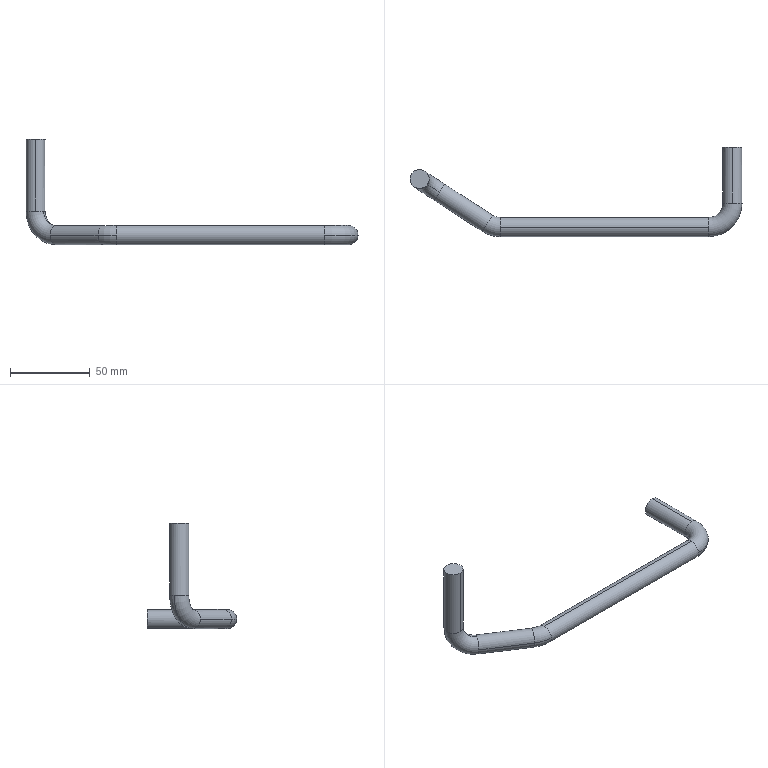Part | SolidWorks | features 3DProfileFeature 2, Sweep 1 | 1 solid | 16 faces | box 208.199 x 56 x 66 mm | volume 34151 mm3 | cylinder 8 | torus 6 | plane 2 | commonest cylinder face diameters 12 x8
STEP:
#1=CARTESIAN_POINT('',(-33.619,21.831,-6.));
#2=VERTEX_POINT('',#1);
#3=CARTESIAN_POINT('',(-30.351,26.863,0.));
#4=VERTEX_POINT('',#3);
#5=CARTESIAN_POINT('',(-33.619,21.831,0.));
#6=DIRECTION('',(0.8387,-0.5446,0.));
#7=DIRECTION('',(0.4568,0.7034,-0.5446));
#8=AXIS2_PLACEMENT_3D('',#5,#6,#7);
#9=CIRCLE('',#8,6.);
#10=EDGE_CURVE('',#2,#4,#9,.T.);
#11=ORIENTED_EDGE('',*,*,#10,.F.);
#12=CARTESIAN_POINT('',(-51.231,33.268,15.));
#13=VERTEX_POINT('',#12);
#14=CARTESIAN_POINT('',(-33.619,21.831,15.));
#15=DIRECTION('',(0.5446,0.8387,0.));
#16=DIRECTION('',(-0.8387,0.5446,0.));
#17=AXIS2_PLACEMENT_3D('',#14,#15,#16);
#18=CIRCLE('',#17,21.);
#19=EDGE_CURVE('',#2,#13,#18,.T.);
#20=ORIENTED_EDGE('',*,*,#19,.T.);
#21=CARTESIAN_POINT('',(-46.199,36.,15.));
#22=VERTEX_POINT('',#21);
#23=CARTESIAN_POINT('',(-46.199,30.,15.));
#24=DIRECTION('',(0.,0.,-1.));
#25=DIRECTION('',(0.,1.,0.));
#26=AXIS2_PLACEMENT_3D('',#23,#24,#25);
#27=CIRCLE('',#26,6.);
#28=EDGE_CURVE('',#13,#22,#27,.T.);
#29=ORIENTED_EDGE('',*,*,#28,.T.);
#30=CARTESIAN_POINT('',(-41.167,26.732,15.));
#31=VERTEX_POINT('',#30);
#32=CARTESIAN_POINT('',(-46.199,30.,15.));
#33=DIRECTION('',(0.,0.,-1.));
#34=DIRECTION('',(0.,1.,0.));
#35=AXIS2_PLACEMENT_3D('',#32,#33,#34);
#36=CIRCLE('',#35,6.);
#37=EDGE_CURVE('',#22,#31,#36,.T.);
#38=ORIENTED_EDGE('',*,*,#37,.T.);
#39=CARTESIAN_POINT('',(-33.619,21.831,6.));
#40=VERTEX_POINT('',#39);
#41=CARTESIAN_POINT('',(-33.619,21.831,15.));
#42=DIRECTION('',(0.5446,0.8387,0.));
#43=DIRECTION('',(-0.8387,0.5446,0.));
#44=AXIS2_PLACEMENT_3D('',#41,#42,#43);
#45=CIRCLE('',#44,9.);
#46=EDGE_CURVE('',#40,#31,#45,.T.);
#47=ORIENTED_EDGE('',*,*,#46,.F.);
#48=CARTESIAN_POINT('',(-33.619,21.831,0.));
#49=DIRECTION('',(0.8387,-0.5446,0.));
#50=DIRECTION('',(0.4568,0.7034,-0.5446));
#51=AXIS2_PLACEMENT_3D('',#48,#49,#50);
#52=CIRCLE('',#51,6.);
#53=EDGE_CURVE('',#4,#40,#52,.T.);
#54=ORIENTED_EDGE('',*,*,#53,.F.);
#55=EDGE_LOOP('',(#11,#20,#29,#38,#47,#54));
#56=FACE_OUTER_BOUND('',#55,.T.);
#57=CARTESIAN_POINT('',(-33.619,21.831,15.));
#58=DIRECTION('',(0.5446,0.8387,0.));
#59=DIRECTION('',(-0.8387,0.5446,0.));
#60=AXIS2_PLACEMENT_3D('',#57,#58,#59);
#61=TOROIDAL_SURFACE('',#60,15.,6.);
#62=ADVANCED_FACE('',(#56),#61,.T.);
#63=CARTESIAN_POINT('',(4.443,-6.,0.));
#64=VERTEX_POINT('',#63);
#65=CARTESIAN_POINT('',(4.443,0.,-6.));
#66=VERTEX_POINT('',#65);
#67=CARTESIAN_POINT('',(4.443,0.,0.));
#68=DIRECTION('',(1.,0.,0.));
#69=DIRECTION('',(0.,0.8387,-0.5446));
#70=AXIS2_PLACEMENT_3D('',#67,#68,#69);
#71=CIRCLE('',#70,6.);
#72=EDGE_CURVE('',#64,#66,#71,.T.);
#73=ORIENTED_EDGE('',*,*,#72,.F.);
#74=CARTESIAN_POINT('',(-6.994,-2.612,0.));
#75=VERTEX_POINT('',#74);
#76=CARTESIAN_POINT('',(4.443,15.,0.));
#77=DIRECTION('',(0.,0.,-1.));
#78=DIRECTION('',(-1.,0.,0.));
#79=AXIS2_PLACEMENT_3D('',#76,#77,#78);
#80=CIRCLE('',#79,21.);
#81=EDGE_CURVE('',#64,#75,#80,.T.);
#82=ORIENTED_EDGE('',*,*,#81,.T.);
#83=CARTESIAN_POINT('',(-0.4586,7.452,0.));
#84=VERTEX_POINT('',#83);
#85=CARTESIAN_POINT('',(-3.726,2.42,0.));
#86=DIRECTION('',(0.8387,-0.5446,0.));
#87=DIRECTION('',(0.4568,0.7034,-0.5446));
#88=AXIS2_PLACEMENT_3D('',#85,#86,#87);
#89=CIRCLE('',#88,6.);
#90=EDGE_CURVE('',#75,#84,#89,.T.);
#91=ORIENTED_EDGE('',*,*,#90,.T.);
#92=CARTESIAN_POINT('',(4.443,6.,0.));
#93=VERTEX_POINT('',#92);
#94=CARTESIAN_POINT('',(4.443,15.,0.));
#95=DIRECTION('',(0.,0.,-1.));
#96=DIRECTION('',(-1.,0.,0.));
#97=AXIS2_PLACEMENT_3D('',#94,#95,#96);
#98=CIRCLE('',#97,9.);
#99=EDGE_CURVE('',#93,#84,#98,.T.);
#100=ORIENTED_EDGE('',*,*,#99,.F.);
#101=CARTESIAN_POINT('',(4.443,0.,0.));
#102=DIRECTION('',(1.,0.,0.));
#103=DIRECTION('',(0.,0.8387,-0.5446));
#104=AXIS2_PLACEMENT_3D('',#101,#102,#103);
#105=CIRCLE('',#104,6.);
#106=EDGE_CURVE('',#66,#93,#105,.T.);
#107=ORIENTED_EDGE('',*,*,#106,.F.);
#108=EDGE_LOOP('',(#73,#82,#91,#100,#107));
#109=FACE_OUTER_BOUND('',#108,.T.);
#110=CARTESIAN_POINT('',(4.443,15.,0.));
#111=DIRECTION('',(0.,0.,-1.));
#112=DIRECTION('',(-1.,0.,0.));
#113=AXIS2_PLACEMENT_3D('',#110,#111,#112);
#114=TOROIDAL_SURFACE('',#113,15.,6.);
#115=ADVANCED_FACE('',(#109),#114,.T.);
#116=CARTESIAN_POINT('',(156.,15.,0.));
#117=VERTEX_POINT('',#116);
#118=CARTESIAN_POINT('',(150.,15.,-6.));
#119=VERTEX_POINT('',#118);
#120=CARTESIAN_POINT('',(150.,15.,0.));
#121=DIRECTION('',(0.,1.,0.));
#122=DIRECTION('',(-0.8387,0.,-0.5446));
#123=AXIS2_PLACEMENT_3D('',#120,#121,#122);
#124=CIRCLE('',#123,6.);
#125=EDGE_CURVE('',#117,#119,#124,.T.);
#126=ORIENTED_EDGE('',*,*,#125,.F.);
#127=CARTESIAN_POINT('',(135.,-6.,0.));
#128=VERTEX_POINT('',#127);
#129=CARTESIAN_POINT('',(135.,15.,0.));
#130=DIRECTION('',(0.,0.,-1.));
#131=DIRECTION('',(-1.,0.,0.));
#132=AXIS2_PLACEMENT_3D('',#129,#130,#131);
#133=CIRCLE('',#132,21.);
#134=EDGE_CURVE('',#117,#128,#133,.T.);
#135=ORIENTED_EDGE('',*,*,#134,.T.);
#136=CARTESIAN_POINT('',(135.,0.,-6.));
#137=VERTEX_POINT('',#136);
#138=CARTESIAN_POINT('',(135.,0.,0.));
#139=DIRECTION('',(1.,0.,0.));
#140=DIRECTION('',(0.,0.8387,-0.5446));
#141=AXIS2_PLACEMENT_3D('',#138,#139,#140);
#142=CIRCLE('',#141,6.);
#143=EDGE_CURVE('',#128,#137,#142,.T.);
#144=ORIENTED_EDGE('',*,*,#143,.T.);
#145=CARTESIAN_POINT('',(135.,6.,0.));
#146=VERTEX_POINT('',#145);
#147=CARTESIAN_POINT('',(135.,0.,0.));
#148=DIRECTION('',(1.,0.,0.));
#149=DIRECTION('',(0.,0.8387,-0.5446));
#150=AXIS2_PLACEMENT_3D('',#147,#148,#149);
#151=CIRCLE('',#150,6.);
#152=EDGE_CURVE('',#137,#146,#151,.T.);
#153=ORIENTED_EDGE('',*,*,#152,.T.);
#154=CARTESIAN_POINT('',(144.,15.,0.));
#155=VERTEX_POINT('',#154);
#156=CARTESIAN_POINT('',(135.,15.,0.));
#157=DIRECTION('',(0.,0.,-1.));
#158=DIRECTION('',(-1.,0.,0.));
#159=AXIS2_PLACEMENT_3D('',#156,#157,#158);
#160=CIRCLE('',#159,9.);
#161=EDGE_CURVE('',#155,#146,#160,.T.);
#162=ORIENTED_EDGE('',*,*,#161,.F.);
#163=CARTESIAN_POINT('',(150.,15.,0.));
#164=DIRECTION('',(0.,1.,0.));
#165=DIRECTION('',(-0.8387,0.,-0.5446));
#166=AXIS2_PLACEMENT_3D('',#163,#164,#165);
#167=CIRCLE('',#166,6.);
#168=EDGE_CURVE('',#119,#155,#167,.T.);
#169=ORIENTED_EDGE('',*,*,#168,.F.);
#170=EDGE_LOOP('',(#126,#135,#144,#153,#162,#169));
#171=FACE_OUTER_BOUND('',#170,.T.);
#172=CARTESIAN_POINT('',(135.,15.,0.));
#173=DIRECTION('',(0.,0.,-1.));
#174=DIRECTION('',(-1.,0.,0.));
#175=AXIS2_PLACEMENT_3D('',#172,#173,#174);
#176=TOROIDAL_SURFACE('',#175,15.,6.);
#177=ADVANCED_FACE('',(#171),#176,.T.);
#178=ORIENTED_EDGE('',*,*,#37,.F.);
#179=CARTESIAN_POINT('',(-46.199,36.,60.));
#180=VERTEX_POINT('',#179);
#181=CARTESIAN_POINT('',(-46.199,36.,15.));
#182=DIRECTION('',(0.,0.,1.));
#183=VECTOR('',#182,1000.);
#184=LINE('',#181,#183);
#185=EDGE_CURVE('',#22,#180,#184,.T.);
#186=ORIENTED_EDGE('',*,*,#185,.T.);
#187=CARTESIAN_POINT('',(-46.199,24.,60.));
#188=VERTEX_POINT('',#187);
#189=CARTESIAN_POINT('',(-46.199,30.,60.));
#190=DIRECTION('',(0.,0.,-1.));
#191=DIRECTION('',(0.,1.,0.));
#192=AXIS2_PLACEMENT_3D('',#189,#190,#191);
#193=CIRCLE('',#192,6.);
#194=EDGE_CURVE('',#180,#188,#193,.T.);
#195=ORIENTED_EDGE('',*,*,#194,.T.);
#196=CARTESIAN_POINT('',(-46.199,24.,15.));
#197=VERTEX_POINT('',#196);
#198=CARTESIAN_POINT('',(-46.199,24.,15.));
#199=DIRECTION('',(0.,0.,1.));
#200=VECTOR('',#199,1000.);
#201=LINE('',#198,#200);
#202=EDGE_CURVE('',#197,#188,#201,.T.);
#203=ORIENTED_EDGE('',*,*,#202,.F.);
#204=CARTESIAN_POINT('',(-46.199,30.,15.));
#205=DIRECTION('',(0.,0.,-1.));
#206=DIRECTION('',(0.,1.,0.));
#207=AXIS2_PLACEMENT_3D('',#204,#205,#206);
#208=CIRCLE('',#207,6.);
#209=EDGE_CURVE('',#31,#197,#208,.T.);
#210=ORIENTED_EDGE('',*,*,#209,.F.);
#211=EDGE_LOOP('',(#178,#186,#195,#203,#210));
#212=FACE_OUTER_BOUND('',#211,.T.);
#213=CARTESIAN_POINT('',(-46.199,30.,15.));
#214=DIRECTION('',(0.,0.,1.));
#215=DIRECTION('',(0.,-1.,0.));
#216=AXIS2_PLACEMENT_3D('',#213,#214,#215);
#217=CYLINDRICAL_SURFACE('',#216,6.);
#218=ADVANCED_FACE('',(#212),#217,.T.);
#219=CARTESIAN_POINT('',(-3.726,2.42,0.));
#220=DIRECTION('',(0.8387,-0.5446,0.));
#221=DIRECTION('',(0.4568,0.7034,-0.5446));
#222=AXIS2_PLACEMENT_3D('',#219,#220,#221);
#223=CIRCLE('',#222,6.);
#224=EDGE_CURVE('',#84,#75,#223,.T.);
#225=ORIENTED_EDGE('',*,*,#224,.F.);
#226=CARTESIAN_POINT('',(-0.4586,7.452,0.));
#227=DIRECTION('',(-0.8387,0.5446,0.));
#228=VECTOR('',#227,1000.);
#229=LINE('',#226,#228);
#230=EDGE_CURVE('',#84,#4,#229,.T.);
#231=ORIENTED_EDGE('',*,*,#230,.T.);
#232=ORIENTED_EDGE('',*,*,#53,.T.);
#233=CARTESIAN_POINT('',(-36.887,16.799,0.));
#234=VERTEX_POINT('',#233);
#235=CARTESIAN_POINT('',(-33.619,21.831,0.));
#236=DIRECTION('',(0.8387,-0.5446,0.));
#237=DIRECTION('',(0.4568,0.7034,-0.5446));
#238=AXIS2_PLACEMENT_3D('',#235,#236,#237);
#239=CIRCLE('',#238,6.);
#240=EDGE_CURVE('',#40,#234,#239,.T.);
#241=ORIENTED_EDGE('',*,*,#240,.T.);
#242=CARTESIAN_POINT('',(-6.994,-2.612,0.));
#243=DIRECTION('',(-0.8387,0.5446,0.));
#244=VECTOR('',#243,1000.);
#245=LINE('',#242,#244);
#246=EDGE_CURVE('',#75,#234,#245,.T.);
#247=ORIENTED_EDGE('',*,*,#246,.F.);
#248=EDGE_LOOP('',(#225,#231,#232,#241,#247));
#249=FACE_OUTER_BOUND('',#248,.T.);
#250=CARTESIAN_POINT('',(-3.726,2.42,0.));
#251=DIRECTION('',(-0.8387,0.5446,0.));
#252=DIRECTION('',(-0.5446,-0.8387,0.));
#253=AXIS2_PLACEMENT_3D('',#250,#251,#252);
#254=CYLINDRICAL_SURFACE('',#253,6.);
#255=ADVANCED_FACE('',(#249),#254,.T.);
#256=ORIENTED_EDGE('',*,*,#152,.F.);
#257=CARTESIAN_POINT('',(135.,0.,-6.));
#258=DIRECTION('',(-1.,0.,0.));
#259=VECTOR('',#258,1000.);
#260=LINE('',#257,#259);
#261=EDGE_CURVE('',#137,#66,#260,.T.);
#262=ORIENTED_EDGE('',*,*,#261,.T.);
#263=ORIENTED_EDGE('',*,*,#106,.T.);
#264=CARTESIAN_POINT('',(4.443,0.,6.));
#265=VERTEX_POINT('',#264);
#266=CARTESIAN_POINT('',(4.443,0.,0.));
#267=DIRECTION('',(1.,0.,0.));
#268=DIRECTION('',(0.,0.8387,-0.5446));
#269=AXIS2_PLACEMENT_3D('',#266,#267,#268);
#270=CIRCLE('',#269,6.);
#271=EDGE_CURVE('',#93,#265,#270,.T.);
#272=ORIENTED_EDGE('',*,*,#271,.T.);
#273=CARTESIAN_POINT('',(135.,0.,6.));
#274=VERTEX_POINT('',#273);
#275=CARTESIAN_POINT('',(135.,0.,6.));
#276=DIRECTION('',(-1.,0.,0.));
#277=VECTOR('',#276,1000.);
#278=LINE('',#275,#277);
#279=EDGE_CURVE('',#274,#265,#278,.T.);
#280=ORIENTED_EDGE('',*,*,#279,.F.);
#281=CARTESIAN_POINT('',(135.,0.,0.));
#282=DIRECTION('',(1.,0.,0.));
#283=DIRECTION('',(0.,0.8387,-0.5446));
#284=AXIS2_PLACEMENT_3D('',#281,#282,#283);
#285=CIRCLE('',#284,6.);
#286=EDGE_CURVE('',#146,#274,#285,.T.);
#287=ORIENTED_EDGE('',*,*,#286,.F.);
#288=EDGE_LOOP('',(#256,#262,#263,#272,#280,#287));
#289=FACE_OUTER_BOUND('',#288,.T.);
#290=CARTESIAN_POINT('',(135.,0.,0.));
#291=DIRECTION('',(-1.,0.,0.));
#292=DIRECTION('',(0.,0.,1.));
#293=AXIS2_PLACEMENT_3D('',#290,#291,#292);
#294=CYLINDRICAL_SURFACE('',#293,6.);
#295=ADVANCED_FACE('',(#289),#294,.T.);
#296=CARTESIAN_POINT('',(150.,50.,6.));
#297=VERTEX_POINT('',#296);
#298=CARTESIAN_POINT('',(150.,50.,-6.));
#299=VERTEX_POINT('',#298);
#300=CARTESIAN_POINT('',(150.,50.,0.));
#301=DIRECTION('',(0.,1.,0.));
#302=DIRECTION('',(-0.8387,0.,-0.5446));
#303=AXIS2_PLACEMENT_3D('',#300,#301,#302);
#304=CIRCLE('',#303,6.);
#305=EDGE_CURVE('',#297,#299,#304,.T.);
#306=ORIENTED_EDGE('',*,*,#305,.F.);
#307=CARTESIAN_POINT('',(150.,15.,6.));
#308=VERTEX_POINT('',#307);
#309=CARTESIAN_POINT('',(150.,50.,6.));
#310=DIRECTION('',(0.,-1.,0.));
#311=VECTOR('',#310,1000.);
#312=LINE('',#309,#311);
#313=EDGE_CURVE('',#297,#308,#312,.T.);
#314=ORIENTED_EDGE('',*,*,#313,.T.);
#315=CARTESIAN_POINT('',(150.,15.,0.));
#316=DIRECTION('',(0.,1.,0.));
#317=DIRECTION('',(-0.8387,0.,-0.5446));
#318=AXIS2_PLACEMENT_3D('',#315,#316,#317);
#319=CIRCLE('',#318,6.);
#320=EDGE_CURVE('',#308,#117,#319,.T.);
#321=ORIENTED_EDGE('',*,*,#320,.T.);
#322=ORIENTED_EDGE('',*,*,#125,.T.);
#323=CARTESIAN_POINT('',(150.,50.,-6.));
#324=DIRECTION('',(0.,-1.,0.));
#325=VECTOR('',#324,1000.);
#326=LINE('',#323,#325);
#327=EDGE_CURVE('',#299,#119,#326,.T.);
#328=ORIENTED_EDGE('',*,*,#327,.F.);
#329=EDGE_LOOP('',(#306,#314,#321,#322,#328));
#330=FACE_OUTER_BOUND('',#329,.T.);
#331=CARTESIAN_POINT('',(150.,50.,0.));
#332=DIRECTION('',(0.,-1.,0.));
#333=DIRECTION('',(0.,0.,-1.));
#334=AXIS2_PLACEMENT_3D('',#331,#332,#333);
#335=CYLINDRICAL_SURFACE('',#334,6.);
#336=ADVANCED_FACE('',(#330),#335,.T.);
#337=ORIENTED_EDGE('',*,*,#185,.F.);
#338=ORIENTED_EDGE('',*,*,#28,.F.);
#339=CARTESIAN_POINT('',(-46.199,30.,15.));
#340=DIRECTION('',(0.,0.,-1.));
#341=DIRECTION('',(0.,1.,0.));
#342=AXIS2_PLACEMENT_3D('',#339,#340,#341);
#343=CIRCLE('',#342,6.);
#344=EDGE_CURVE('',#197,#13,#343,.T.);
#345=ORIENTED_EDGE('',*,*,#344,.F.);
#346=ORIENTED_EDGE('',*,*,#202,.T.);
#347=CARTESIAN_POINT('',(-46.199,30.,60.));
#348=DIRECTION('',(0.,0.,-1.));
#349=DIRECTION('',(0.,1.,0.));
#350=AXIS2_PLACEMENT_3D('',#347,#348,#349);
#351=CIRCLE('',#350,6.);
#352=EDGE_CURVE('',#188,#180,#351,.T.);
#353=ORIENTED_EDGE('',*,*,#352,.T.);
#354=EDGE_LOOP('',(#337,#338,#345,#346,#353));
#355=FACE_OUTER_BOUND('',#354,.T.);
#356=CARTESIAN_POINT('',(-46.199,30.,15.));
#357=DIRECTION('',(0.,0.,1.));
#358=DIRECTION('',(0.,-1.,0.));
#359=AXIS2_PLACEMENT_3D('',#356,#357,#358);
#360=CYLINDRICAL_SURFACE('',#359,6.);
#361=ADVANCED_FACE('',(#355),#360,.T.);
#362=ORIENTED_EDGE('',*,*,#19,.F.);
#363=CARTESIAN_POINT('',(-33.619,21.831,0.));
#364=DIRECTION('',(0.8387,-0.5446,0.));
#365=DIRECTION('',(0.4568,0.7034,-0.5446));
#366=AXIS2_PLACEMENT_3D('',#363,#364,#365);
#367=CIRCLE('',#366,6.);
#368=EDGE_CURVE('',#234,#2,#367,.T.);
#369=ORIENTED_EDGE('',*,*,#368,.F.);
#370=ORIENTED_EDGE('',*,*,#240,.F.);
#371=ORIENTED_EDGE('',*,*,#46,.T.);
#372=ORIENTED_EDGE('',*,*,#209,.T.);
#373=ORIENTED_EDGE('',*,*,#344,.T.);
#374=EDGE_LOOP('',(#362,#369,#370,#371,#372,#373));
#375=FACE_OUTER_BOUND('',#374,.T.);
#376=CARTESIAN_POINT('',(-33.619,21.831,15.));
#377=DIRECTION('',(0.5446,0.8387,0.));
#378=DIRECTION('',(-0.8387,0.5446,0.));
#379=AXIS2_PLACEMENT_3D('',#376,#377,#378);
#380=TOROIDAL_SURFACE('',#379,15.,6.);
#381=ADVANCED_FACE('',(#375),#380,.T.);
#382=ORIENTED_EDGE('',*,*,#230,.F.);
#383=ORIENTED_EDGE('',*,*,#90,.F.);
#384=ORIENTED_EDGE('',*,*,#246,.T.);
#385=ORIENTED_EDGE('',*,*,#368,.T.);
#386=ORIENTED_EDGE('',*,*,#10,.T.);
#387=EDGE_LOOP('',(#382,#383,#384,#385,#386));
#388=FACE_OUTER_BOUND('',#387,.T.);
#389=CARTESIAN_POINT('',(-3.726,2.42,0.));
#390=DIRECTION('',(-0.8387,0.5446,0.));
#391=DIRECTION('',(-0.5446,-0.8387,0.));
#392=AXIS2_PLACEMENT_3D('',#389,#390,#391);
#393=CYLINDRICAL_SURFACE('',#392,6.);
#394=ADVANCED_FACE('',(#388),#393,.T.);
#395=ORIENTED_EDGE('',*,*,#81,.F.);
#396=CARTESIAN_POINT('',(4.443,0.,0.));
#397=DIRECTION('',(1.,0.,0.));
#398=DIRECTION('',(0.,0.8387,-0.5446));
#399=AXIS2_PLACEMENT_3D('',#396,#397,#398);
#400=CIRCLE('',#399,6.);
#401=EDGE_CURVE('',#265,#64,#400,.T.);
#402=ORIENTED_EDGE('',*,*,#401,.F.);
#403=ORIENTED_EDGE('',*,*,#271,.F.);
#404=ORIENTED_EDGE('',*,*,#99,.T.);
#405=ORIENTED_EDGE('',*,*,#224,.T.);
#406=EDGE_LOOP('',(#395,#402,#403,#404,#405));
#407=FACE_OUTER_BOUND('',#406,.T.);
#408=CARTESIAN_POINT('',(4.443,15.,0.));
#409=DIRECTION('',(0.,0.,-1.));
#410=DIRECTION('',(-1.,0.,0.));
#411=AXIS2_PLACEMENT_3D('',#408,#409,#410);
#412=TOROIDAL_SURFACE('',#411,15.,6.);
#413=ADVANCED_FACE('',(#407),#412,.T.);
#414=ORIENTED_EDGE('',*,*,#261,.F.);
#415=ORIENTED_EDGE('',*,*,#143,.F.);
#416=CARTESIAN_POINT('',(135.,0.,0.));
#417=DIRECTION('',(1.,0.,0.));
#418=DIRECTION('',(0.,0.8387,-0.5446));
#419=AXIS2_PLACEMENT_3D('',#416,#417,#418);
#420=CIRCLE('',#419,6.);
#421=EDGE_CURVE('',#274,#128,#420,.T.);
#422=ORIENTED_EDGE('',*,*,#421,.F.);
#423=ORIENTED_EDGE('',*,*,#279,.T.);
#424=ORIENTED_EDGE('',*,*,#401,.T.);
#425=ORIENTED_EDGE('',*,*,#72,.T.);
#426=EDGE_LOOP('',(#414,#415,#422,#423,#424,#425));
#427=FACE_OUTER_BOUND('',#426,.T.);
#428=CARTESIAN_POINT('',(135.,0.,0.));
#429=DIRECTION('',(-1.,0.,0.));
#430=DIRECTION('',(0.,0.,1.));
#431=AXIS2_PLACEMENT_3D('',#428,#429,#430);
#432=CYLINDRICAL_SURFACE('',#431,6.);
#433=ADVANCED_FACE('',(#427),#432,.T.);
#434=ORIENTED_EDGE('',*,*,#134,.F.);
#435=ORIENTED_EDGE('',*,*,#320,.F.);
#436=CARTESIAN_POINT('',(150.,15.,0.));
#437=DIRECTION('',(0.,1.,0.));
#438=DIRECTION('',(-0.8387,0.,-0.5446));
#439=AXIS2_PLACEMENT_3D('',#436,#437,#438);
#440=CIRCLE('',#439,6.);
#441=EDGE_CURVE('',#155,#308,#440,.T.);
#442=ORIENTED_EDGE('',*,*,#441,.F.);
#443=ORIENTED_EDGE('',*,*,#161,.T.);
#444=ORIENTED_EDGE('',*,*,#286,.T.);
#445=ORIENTED_EDGE('',*,*,#421,.T.);
#446=EDGE_LOOP('',(#434,#435,#442,#443,#444,#445));
#447=FACE_OUTER_BOUND('',#446,.T.);
#448=CARTESIAN_POINT('',(135.,15.,0.));
#449=DIRECTION('',(0.,0.,-1.));
#450=DIRECTION('',(-1.,0.,0.));
#451=AXIS2_PLACEMENT_3D('',#448,#449,#450);
#452=TOROIDAL_SURFACE('',#451,15.,6.);
#453=ADVANCED_FACE('',(#447),#452,.T.);
#454=ORIENTED_EDGE('',*,*,#313,.F.);
#455=CARTESIAN_POINT('',(150.,50.,0.));
#456=DIRECTION('',(0.,1.,0.));
#457=DIRECTION('',(-0.8387,0.,-0.5446));
#458=AXIS2_PLACEMENT_3D('',#455,#456,#457);
#459=CIRCLE('',#458,6.);
#460=EDGE_CURVE('',#299,#297,#459,.T.);
#461=ORIENTED_EDGE('',*,*,#460,.F.);
#462=ORIENTED_EDGE('',*,*,#327,.T.);
#463=ORIENTED_EDGE('',*,*,#168,.T.);
#464=ORIENTED_EDGE('',*,*,#441,.T.);
#465=EDGE_LOOP('',(#454,#461,#462,#463,#464));
#466=FACE_OUTER_BOUND('',#465,.T.);
#467=CARTESIAN_POINT('',(150.,50.,0.));
#468=DIRECTION('',(0.,-1.,0.));
#469=DIRECTION('',(0.,0.,-1.));
#470=AXIS2_PLACEMENT_3D('',#467,#468,#469);
#471=CYLINDRICAL_SURFACE('',#470,6.);
#472=ADVANCED_FACE('',(#466),#471,.T.);
#473=ORIENTED_EDGE('',*,*,#352,.F.);
#474=ORIENTED_EDGE('',*,*,#194,.F.);
#475=EDGE_LOOP('',(#473,#474));
#476=FACE_OUTER_BOUND('',#475,.T.);
#477=CARTESIAN_POINT('',(-46.199,30.,60.));
#478=DIRECTION('',(0.,0.,-1.));
#479=DIRECTION('',(0.,1.,0.));
#480=AXIS2_PLACEMENT_3D('',#477,#478,#479);
#481=PLANE('',#480);
#482=ADVANCED_FACE('',(#476),#481,.F.);
#483=ORIENTED_EDGE('',*,*,#460,.T.);
#484=ORIENTED_EDGE('',*,*,#305,.T.);
#485=EDGE_LOOP('',(#483,#484));
#486=FACE_OUTER_BOUND('',#485,.T.);
#487=CARTESIAN_POINT('',(150.,50.,0.));
#488=DIRECTION('',(0.,1.,0.));
#489=DIRECTION('',(-0.8387,0.,-0.5446));
#490=AXIS2_PLACEMENT_3D('',#487,#488,#489);
#491=PLANE('',#490);
#492=ADVANCED_FACE('',(#486),#491,.T.);
#493=CLOSED_SHELL('',(#62,#115,#177,#218,#255,#295,#336,#361,#381,#394,#413,#433,#453,#472,#482,#492));
#494=MANIFOLD_SOLID_BREP('',#493);
#495=CARTESIAN_POINT('',(0.,0.,0.));
#496=DIRECTION('',(0.,0.,1.));
#497=DIRECTION('',(1.,0.,0.));
#498=AXIS2_PLACEMENT_3D('',#495,#496,#497);
#499=(LENGTH_UNIT()NAMED_UNIT(*)SI_UNIT(.MILLI.,.METRE.));
#500=UNCERTAINTY_MEASURE_WITH_UNIT(LENGTH_MEASURE(0.00001),#499,'','');
#501=(NAMED_UNIT(*)PLANE_ANGLE_UNIT()SI_UNIT($,.RADIAN.));
#502=(NAMED_UNIT(*)SI_UNIT($,.STERADIAN.)SOLID_ANGLE_UNIT());
#503=(GEOMETRIC_REPRESENTATION_CONTEXT(3)GLOBAL_UNCERTAINTY_ASSIGNED_CONTEXT((#500))GLOBAL_UNIT_ASSIGNED_CONTEXT((#499,#501,#502))REPRESENTATION_CONTEXT('',''));
#504=ADVANCED_BREP_SHAPE_REPRESENTATION('',(#494,#498),#503);